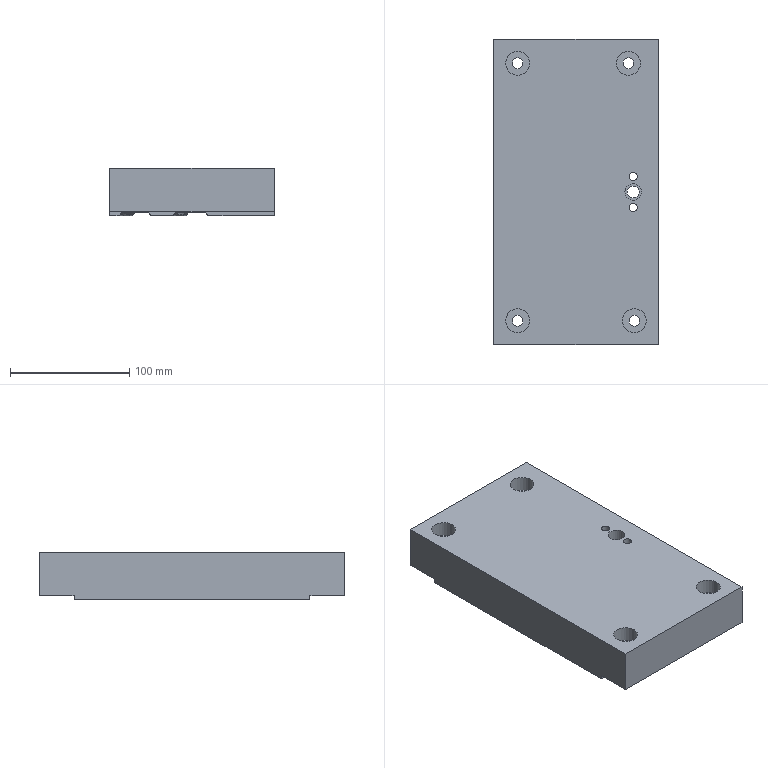Part | NX | features solid 2 | 1 solid | 170 faces | box 138 x 256 x 40 mm | volume 1301824 mm3 | cylinder 64 | spline 47 | plane 29 | torus 26 | cone 4 | commonest cylinder face diameters 4 x23 5 x11 3 x4 6 x4 8.499 x4 9 x4